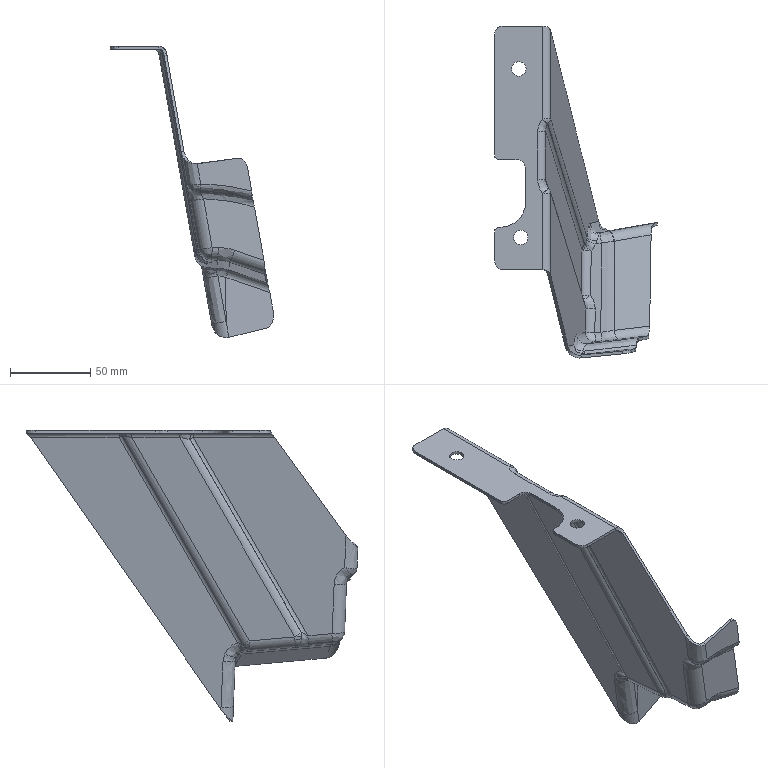Part | 1 solid | 151 faces | box 101.622 x 206.741 x 181.468 mm | volume 54845 mm3 | spline 77 | cylinder 46 | plane 21 | sphere 4 | other 3 | commonest cylinder face diameters 10 x11 6.4 x7 12 x6 15.6 x6 9 x4 13.6 x3